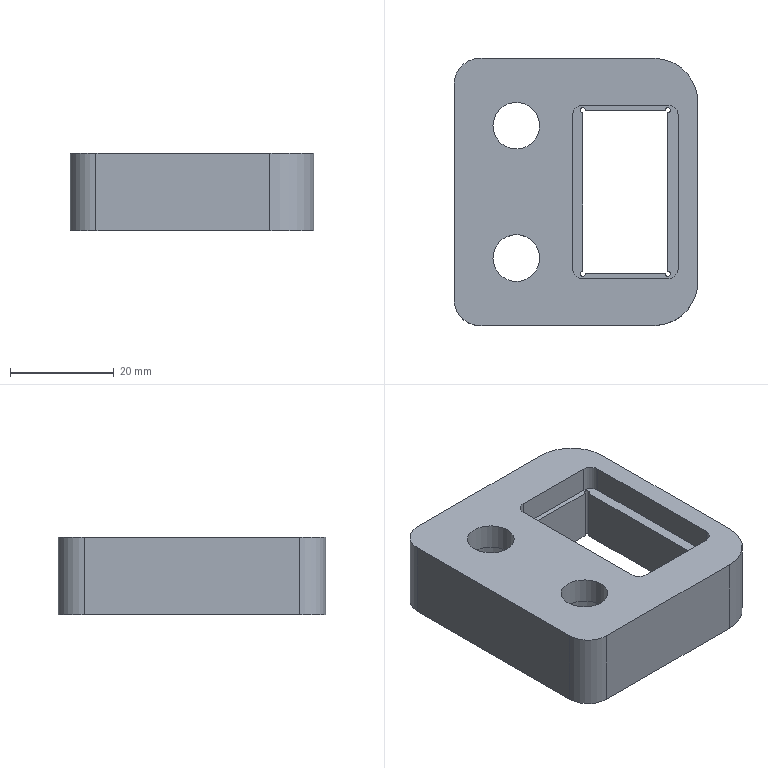Part | STEP file | 434_id1606_x_t | 1 solid | 33 faces | box 47 x 51.5 x 15 mm | volume 23387 mm3 | plane 17 | cylinder 16 | commonest cylinder face diameters 1 x4 4 x4 9 x2 10 x2 14 x2 17 x2